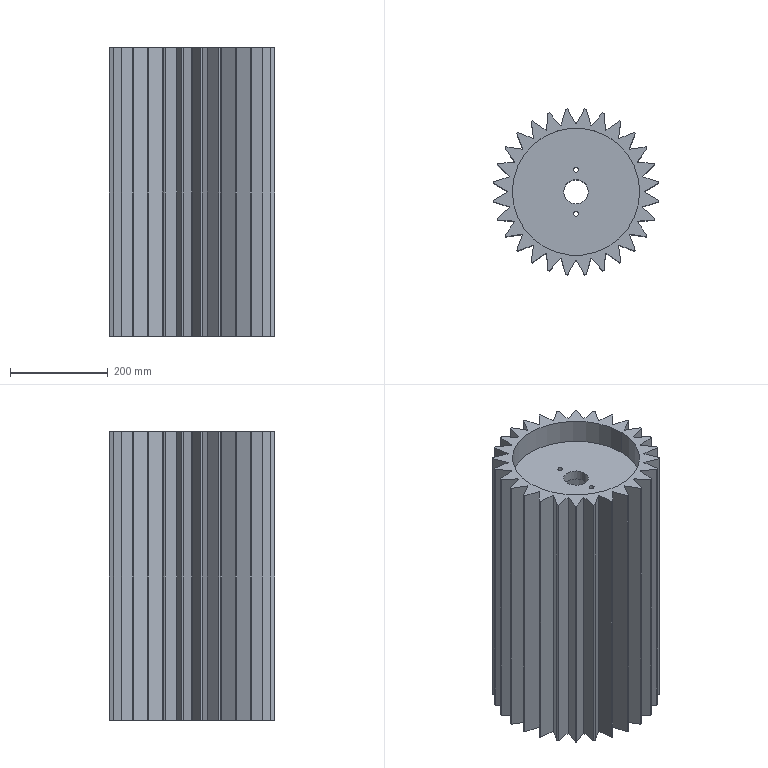Part | SolidWorks | features BaseBody 1, ICE 1 | 1 solid | 136 faces | box 338.194 x 338.194 x 590 mm | volume 24931977 mm3 | plane 90 | cylinder 46 | commonest cylinder face diameters 340 x28 10 x8 50 x4 260 x4 200 x2